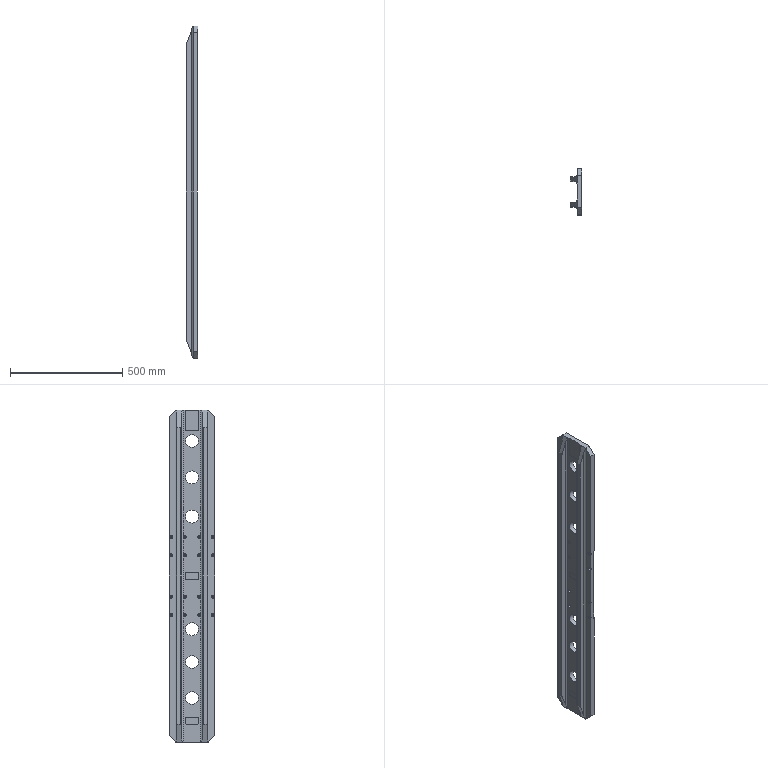Part | Creo | features CURVE 12, CUT 10, DATUM PLANE 3, PROTRUSION 3, ROUND 3, CHAMFER 1, COORDINATE SYSTEM 1, MIRROR 1 | 1 solid | 158 faces | box 53 x 205 x 1480 mm | volume 7789168 mm3 | cylinder 90 | plane 68 | commonest cylinder face diameters 8.5 x32 14 x32 57.474 x12 12 x10 16 x4